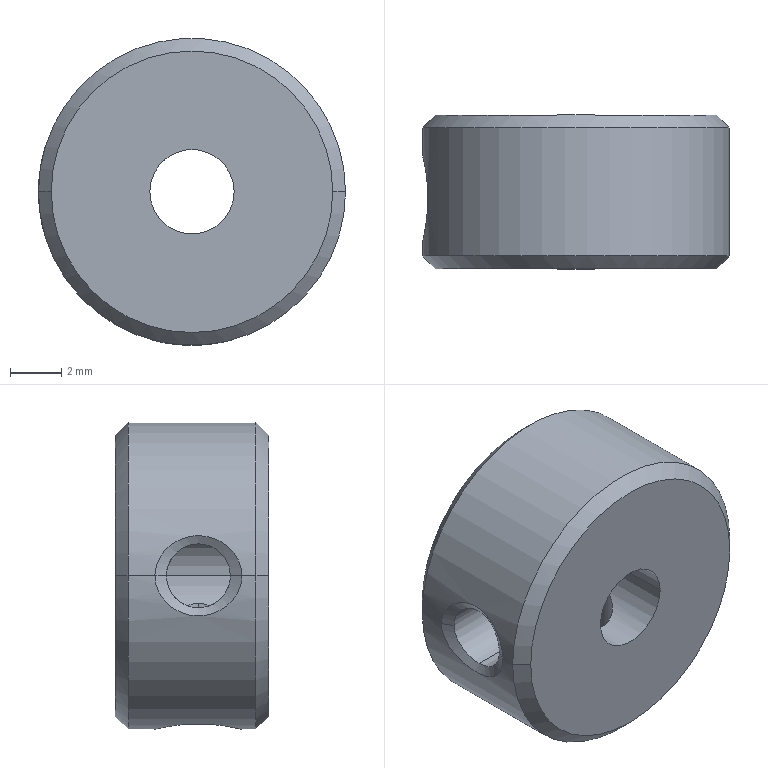Part | NX | 1 solid | 20 faces | box 12 x 6 x 12 mm | volume 572.085 mm3 | cylinder 8 | cone 6 | spline 4 | plane 2 | commonest cylinder face diameters 2.5 x4 3.3 x2 12 x2